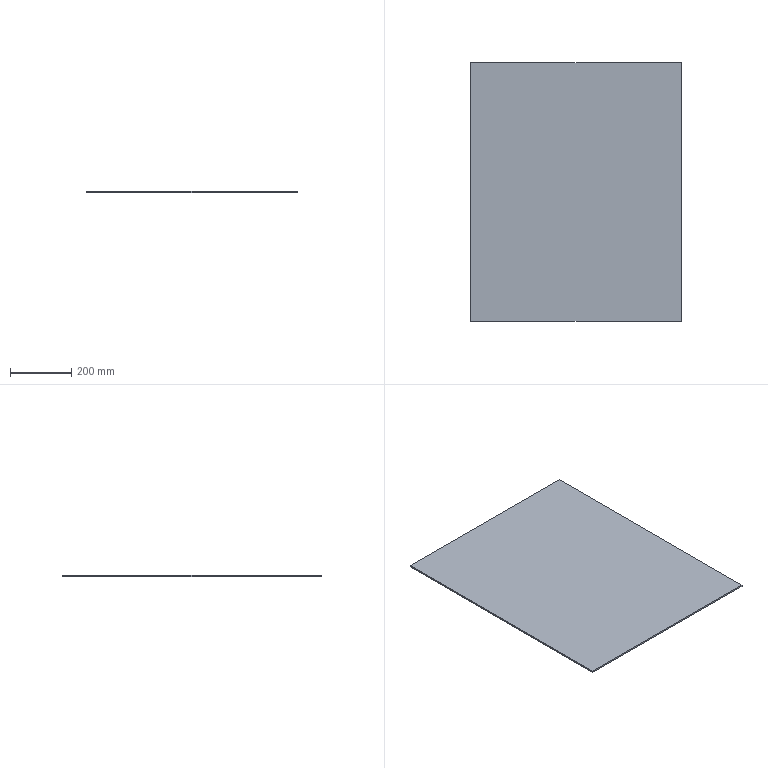Part | SolidWorks | features Extrusion 1, HoleWzd 1 | 1 solid | 6 faces | box 686 x 842 x 5 mm | volume 2888060 mm3 | plane 6
STEP:
#1=CARTESIAN_POINT('',(343.,-421.,0.));
#2=VERTEX_POINT('',#1);
#3=CARTESIAN_POINT('',(343.,421.,0.));
#4=VERTEX_POINT('',#3);
#5=CARTESIAN_POINT('',(343.,421.,0.));
#6=DIRECTION('',(0.,1.,0.));
#7=VECTOR('',#6,1000.);
#8=LINE('',#5,#7);
#9=EDGE_CURVE('',#2,#4,#8,.T.);
#10=ORIENTED_EDGE('',*,*,#9,.T.);
#11=CARTESIAN_POINT('',(343.,421.,5.));
#12=VERTEX_POINT('',#11);
#13=CARTESIAN_POINT('',(343.,421.,5.));
#14=DIRECTION('',(0.,0.,-1.));
#15=VECTOR('',#14,1000.);
#16=LINE('',#13,#15);
#17=EDGE_CURVE('',#12,#4,#16,.T.);
#18=ORIENTED_EDGE('',*,*,#17,.F.);
#19=CARTESIAN_POINT('',(343.,-421.,5.));
#20=VERTEX_POINT('',#19);
#21=CARTESIAN_POINT('',(343.,421.,5.));
#22=DIRECTION('',(0.,1.,0.));
#23=VECTOR('',#22,1000.);
#24=LINE('',#21,#23);
#25=EDGE_CURVE('',#20,#12,#24,.T.);
#26=ORIENTED_EDGE('',*,*,#25,.F.);
#27=CARTESIAN_POINT('',(343.,-421.,5.));
#28=DIRECTION('',(0.,0.,-1.));
#29=VECTOR('',#28,1000.);
#30=LINE('',#27,#29);
#31=EDGE_CURVE('',#20,#2,#30,.T.);
#32=ORIENTED_EDGE('',*,*,#31,.T.);
#33=EDGE_LOOP('',(#10,#18,#26,#32));
#34=FACE_OUTER_BOUND('',#33,.T.);
#35=CARTESIAN_POINT('',(343.,421.,5.));
#36=DIRECTION('',(-1.,0.,0.));
#37=DIRECTION('',(0.,-1.,0.));
#38=AXIS2_PLACEMENT_3D('',#35,#36,#37);
#39=PLANE('',#38);
#40=ADVANCED_FACE('',(#34),#39,.F.);
#41=CARTESIAN_POINT('',(-343.,421.,0.));
#42=VERTEX_POINT('',#41);
#43=CARTESIAN_POINT('',(-343.,421.,0.));
#44=DIRECTION('',(-1.,0.,0.));
#45=VECTOR('',#44,1000.);
#46=LINE('',#43,#45);
#47=EDGE_CURVE('',#4,#42,#46,.T.);
#48=ORIENTED_EDGE('',*,*,#47,.T.);
#49=CARTESIAN_POINT('',(-343.,421.,5.));
#50=VERTEX_POINT('',#49);
#51=CARTESIAN_POINT('',(-343.,421.,5.));
#52=DIRECTION('',(0.,0.,-1.));
#53=VECTOR('',#52,1000.);
#54=LINE('',#51,#53);
#55=EDGE_CURVE('',#50,#42,#54,.T.);
#56=ORIENTED_EDGE('',*,*,#55,.F.);
#57=CARTESIAN_POINT('',(-343.,421.,5.));
#58=DIRECTION('',(-1.,0.,0.));
#59=VECTOR('',#58,1000.);
#60=LINE('',#57,#59);
#61=EDGE_CURVE('',#12,#50,#60,.T.);
#62=ORIENTED_EDGE('',*,*,#61,.F.);
#63=ORIENTED_EDGE('',*,*,#17,.T.);
#64=EDGE_LOOP('',(#48,#56,#62,#63));
#65=FACE_OUTER_BOUND('',#64,.T.);
#66=CARTESIAN_POINT('',(-343.,421.,5.));
#67=DIRECTION('',(0.,-1.,0.));
#68=DIRECTION('',(0.,0.,-1.));
#69=AXIS2_PLACEMENT_3D('',#66,#67,#68);
#70=PLANE('',#69);
#71=ADVANCED_FACE('',(#65),#70,.F.);
#72=CARTESIAN_POINT('',(-343.,-421.,0.));
#73=VERTEX_POINT('',#72);
#74=CARTESIAN_POINT('',(-343.,421.,0.));
#75=DIRECTION('',(0.,-1.,0.));
#76=VECTOR('',#75,1000.);
#77=LINE('',#74,#76);
#78=EDGE_CURVE('',#42,#73,#77,.T.);
#79=ORIENTED_EDGE('',*,*,#78,.T.);
#80=CARTESIAN_POINT('',(-343.,-421.,5.));
#81=VERTEX_POINT('',#80);
#82=CARTESIAN_POINT('',(-343.,-421.,5.));
#83=DIRECTION('',(0.,0.,-1.));
#84=VECTOR('',#83,1000.);
#85=LINE('',#82,#84);
#86=EDGE_CURVE('',#81,#73,#85,.T.);
#87=ORIENTED_EDGE('',*,*,#86,.F.);
#88=CARTESIAN_POINT('',(-343.,421.,5.));
#89=DIRECTION('',(0.,-1.,0.));
#90=VECTOR('',#89,1000.);
#91=LINE('',#88,#90);
#92=EDGE_CURVE('',#50,#81,#91,.T.);
#93=ORIENTED_EDGE('',*,*,#92,.F.);
#94=ORIENTED_EDGE('',*,*,#55,.T.);
#95=EDGE_LOOP('',(#79,#87,#93,#94));
#96=FACE_OUTER_BOUND('',#95,.T.);
#97=CARTESIAN_POINT('',(-343.,421.,5.));
#98=DIRECTION('',(1.,0.,0.));
#99=DIRECTION('',(0.,1.,0.));
#100=AXIS2_PLACEMENT_3D('',#97,#98,#99);
#101=PLANE('',#100);
#102=ADVANCED_FACE('',(#96),#101,.F.);
#103=CARTESIAN_POINT('',(-343.,-421.,0.));
#104=DIRECTION('',(1.,0.,0.));
#105=VECTOR('',#104,1000.);
#106=LINE('',#103,#105);
#107=EDGE_CURVE('',#73,#2,#106,.T.);
#108=ORIENTED_EDGE('',*,*,#107,.T.);
#109=ORIENTED_EDGE('',*,*,#31,.F.);
#110=CARTESIAN_POINT('',(-343.,-421.,5.));
#111=DIRECTION('',(1.,0.,0.));
#112=VECTOR('',#111,1000.);
#113=LINE('',#110,#112);
#114=EDGE_CURVE('',#81,#20,#113,.T.);
#115=ORIENTED_EDGE('',*,*,#114,.F.);
#116=ORIENTED_EDGE('',*,*,#86,.T.);
#117=EDGE_LOOP('',(#108,#109,#115,#116));
#118=FACE_OUTER_BOUND('',#117,.T.);
#119=CARTESIAN_POINT('',(-343.,-421.,5.));
#120=DIRECTION('',(0.,1.,0.));
#121=DIRECTION('',(0.,0.,1.));
#122=AXIS2_PLACEMENT_3D('',#119,#120,#121);
#123=PLANE('',#122);
#124=ADVANCED_FACE('',(#118),#123,.F.);
#125=ORIENTED_EDGE('',*,*,#25,.T.);
#126=ORIENTED_EDGE('',*,*,#61,.T.);
#127=ORIENTED_EDGE('',*,*,#92,.T.);
#128=ORIENTED_EDGE('',*,*,#114,.T.);
#129=EDGE_LOOP('',(#125,#126,#127,#128));
#130=FACE_OUTER_BOUND('',#129,.T.);
#131=CARTESIAN_POINT('',(0.,0.,5.));
#132=DIRECTION('',(0.,0.,1.));
#133=DIRECTION('',(1.,0.,0.));
#134=AXIS2_PLACEMENT_3D('',#131,#132,#133);
#135=PLANE('',#134);
#136=ADVANCED_FACE('',(#130),#135,.T.);
#137=ORIENTED_EDGE('',*,*,#9,.F.);
#138=ORIENTED_EDGE('',*,*,#107,.F.);
#139=ORIENTED_EDGE('',*,*,#78,.F.);
#140=ORIENTED_EDGE('',*,*,#47,.F.);
#141=EDGE_LOOP('',(#137,#138,#139,#140));
#142=FACE_OUTER_BOUND('',#141,.T.);
#143=CARTESIAN_POINT('',(0.,0.,0.));
#144=DIRECTION('',(0.,0.,1.));
#145=DIRECTION('',(1.,0.,0.));
#146=AXIS2_PLACEMENT_3D('',#143,#144,#145);
#147=PLANE('',#146);
#148=ADVANCED_FACE('',(#142),#147,.F.);
#149=CLOSED_SHELL('',(#40,#71,#102,#124,#136,#148));
#150=MANIFOLD_SOLID_BREP('',#149);
#151=CARTESIAN_POINT('',(0.,0.,0.));
#152=DIRECTION('',(0.,0.,1.));
#153=DIRECTION('',(1.,0.,0.));
#154=AXIS2_PLACEMENT_3D('',#151,#152,#153);
#155=(LENGTH_UNIT()NAMED_UNIT(*)SI_UNIT(.MILLI.,.METRE.));
#156=UNCERTAINTY_MEASURE_WITH_UNIT(LENGTH_MEASURE(0.00001),#155,'','');
#157=(NAMED_UNIT(*)PLANE_ANGLE_UNIT()SI_UNIT($,.RADIAN.));
#158=(NAMED_UNIT(*)SI_UNIT($,.STERADIAN.)SOLID_ANGLE_UNIT());
#159=(GEOMETRIC_REPRESENTATION_CONTEXT(3)GLOBAL_UNCERTAINTY_ASSIGNED_CONTEXT((#156))GLOBAL_UNIT_ASSIGNED_CONTEXT((#155,#157,#158))REPRESENTATION_CONTEXT('',''));
#160=ADVANCED_BREP_SHAPE_REPRESENTATION('',(#150,#154),#159);